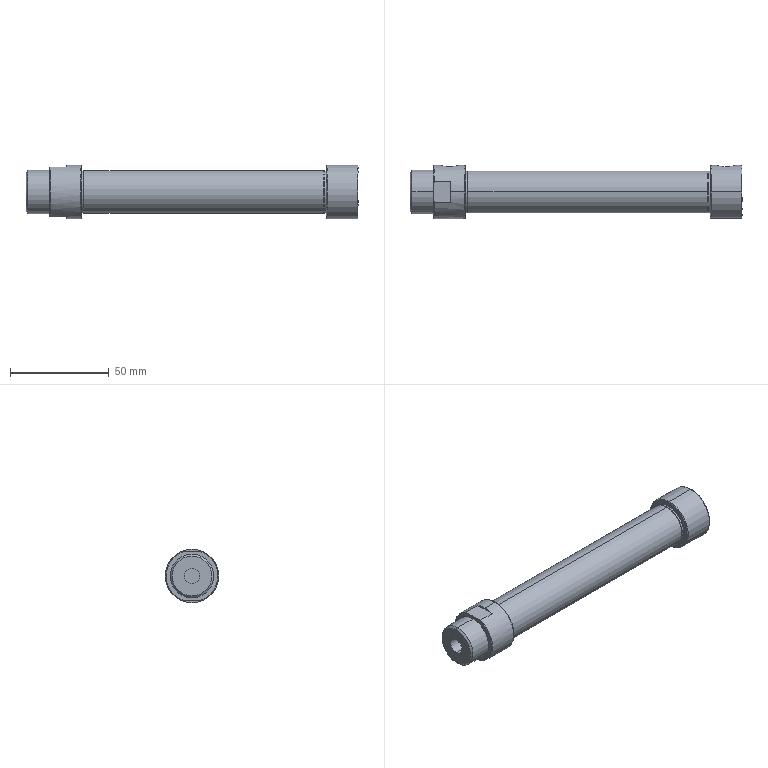Part | STEP file | Copy 1^MA20-80-S-U | 1 solid | 53 faces | box 168 x 27 x 27 mm | volume 32418 mm3 | cylinder 20 | plane 15 | cone 10 | spline 8 | commonest cylinder face diameters 21.4 x6 8.566 x4 27 x4 8 x2 20 x2 22 x2